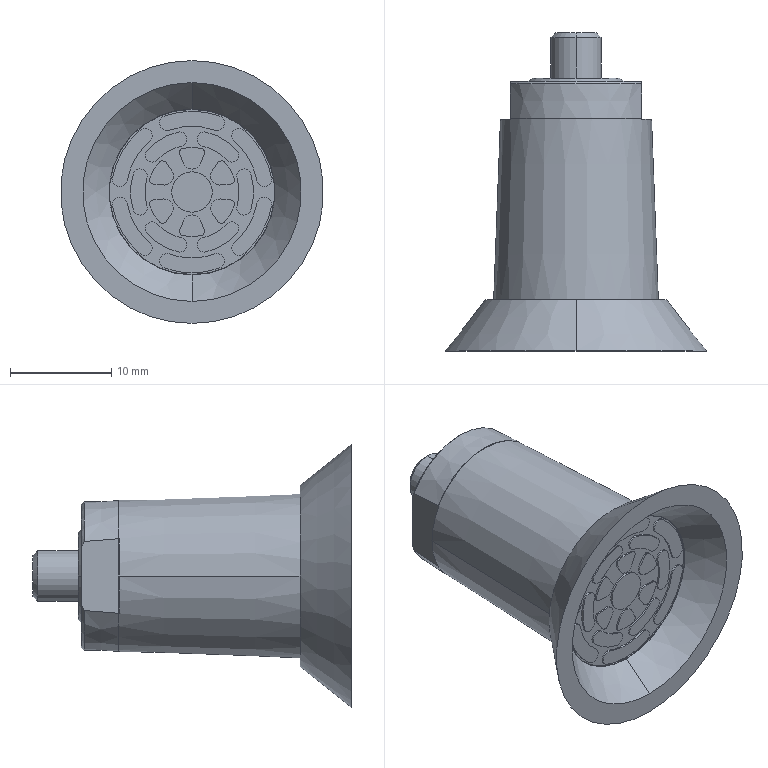Part | SolidWorks | features BaseBody 1 | 1 solid | 161 faces | box 26 x 31.5 x 26 mm | volume 5146 mm3 | cylinder 100 | plane 46 | cone 15 | commonest cylinder face diameters 0.888 x14 1.421 x13 1.464 x11 1.776 x9 1.465 x7 8.432 x7